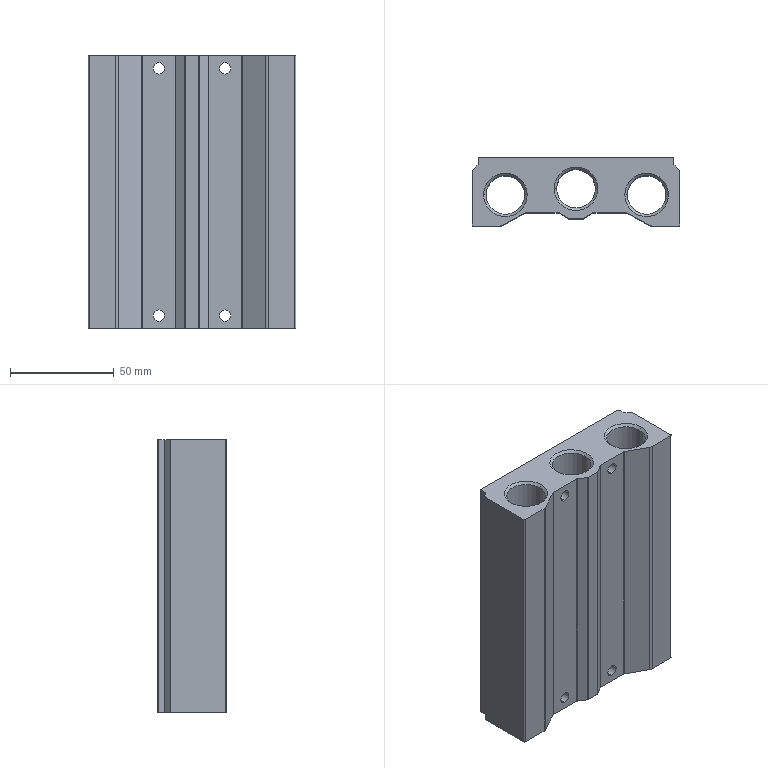Part | STEP file | 400M3F | 1 solid | 112 faces | box 100 x 33 x 131 mm | volume 261917 mm3 | cylinder 58 | cone 36 | plane 18 | commonest cylinder face diameters 1 x12 3.242 x12 12 x12 5.5 x8 14.5 x6 18.631 x6